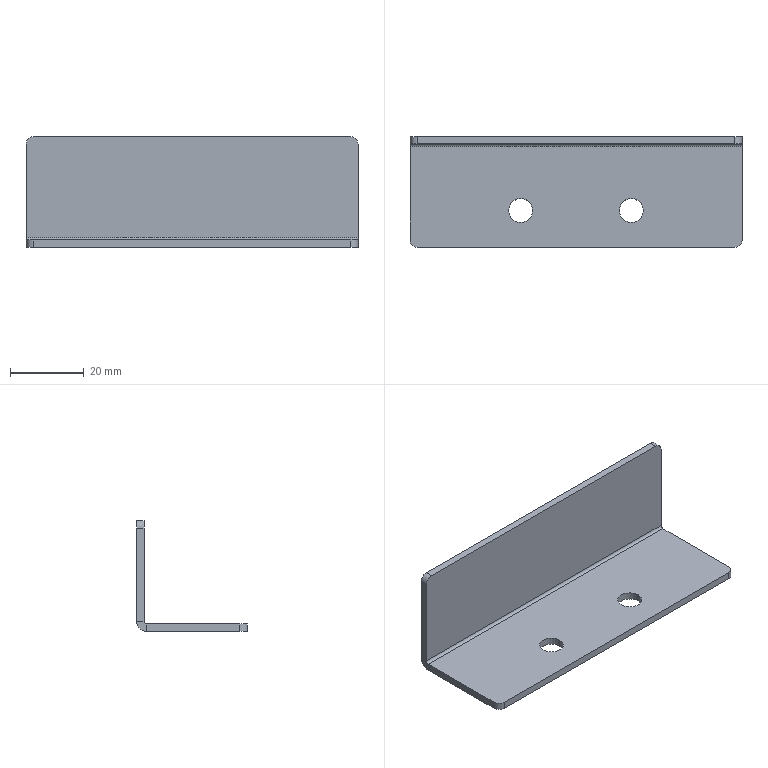Part | STEP file | 02-20 scrap support plate (Default) | 1 solid | 22 faces | box 90 x 30 x 30 mm | volume 10166 mm3 | plane 12 | cylinder 10 | commonest cylinder face diameters 4 x4 6.5 x4 1.473 x1 5.473 x1
STEP:
#1=CARTESIAN_POINT('',(11.75,-4.,-2.));
#2=VERTEX_POINT('',#1);
#3=CARTESIAN_POINT('',(18.25,-4.,-2.));
#4=VERTEX_POINT('',#3);
#5=CARTESIAN_POINT('',(15.,-4.,-2.));
#6=DIRECTION('',(0.,0.,1.));
#7=DIRECTION('',(1.,0.,0.));
#8=AXIS2_PLACEMENT_3D('',#5,#6,#7);
#9=CIRCLE('',#8,3.25);
#10=EDGE_CURVE('',#2,#4,#9,.T.);
#11=ORIENTED_EDGE('',*,*,#10,.F.);
#12=CARTESIAN_POINT('',(11.75,-4.,0.));
#13=VERTEX_POINT('',#12);
#14=CARTESIAN_POINT('',(11.75,-4.,-10.));
#15=DIRECTION('',(0.,0.,1.));
#16=VECTOR('',#15,1000.);
#17=LINE('',#14,#16);
#18=EDGE_CURVE('',#2,#13,#17,.T.);
#19=ORIENTED_EDGE('',*,*,#18,.T.);
#20=CARTESIAN_POINT('',(18.25,-4.,0.));
#21=VERTEX_POINT('',#20);
#22=CARTESIAN_POINT('',(15.,-4.,0.));
#23=DIRECTION('',(0.,0.,1.));
#24=DIRECTION('',(1.,0.,0.));
#25=AXIS2_PLACEMENT_3D('',#22,#23,#24);
#26=CIRCLE('',#25,3.25);
#27=EDGE_CURVE('',#13,#21,#26,.T.);
#28=ORIENTED_EDGE('',*,*,#27,.T.);
#29=CARTESIAN_POINT('',(18.25,-4.,-10.));
#30=DIRECTION('',(0.,0.,1.));
#31=VECTOR('',#30,1000.);
#32=LINE('',#29,#31);
#33=EDGE_CURVE('',#4,#21,#32,.T.);
#34=ORIENTED_EDGE('',*,*,#33,.F.);
#35=EDGE_LOOP('',(#11,#19,#28,#34));
#36=FACE_OUTER_BOUND('',#35,.T.);
#37=CARTESIAN_POINT('',(15.,-4.,-10.));
#38=DIRECTION('',(0.,0.,1.));
#39=DIRECTION('',(1.,0.,0.));
#40=AXIS2_PLACEMENT_3D('',#37,#38,#39);
#41=CYLINDRICAL_SURFACE('',#40,3.25);
#42=ADVANCED_FACE('',(#36),#41,.F.);
#43=CARTESIAN_POINT('',(-18.25,-4.,-2.));
#44=VERTEX_POINT('',#43);
#45=CARTESIAN_POINT('',(-11.75,-4.,-2.));
#46=VERTEX_POINT('',#45);
#47=CARTESIAN_POINT('',(-15.,-4.,-2.));
#48=DIRECTION('',(0.,0.,1.));
#49=DIRECTION('',(1.,0.,0.));
#50=AXIS2_PLACEMENT_3D('',#47,#48,#49);
#51=CIRCLE('',#50,3.25);
#52=EDGE_CURVE('',#44,#46,#51,.T.);
#53=ORIENTED_EDGE('',*,*,#52,.F.);
#54=CARTESIAN_POINT('',(-18.25,-4.,0.));
#55=VERTEX_POINT('',#54);
#56=CARTESIAN_POINT('',(-18.25,-4.,-10.));
#57=DIRECTION('',(0.,0.,1.));
#58=VECTOR('',#57,1000.);
#59=LINE('',#56,#58);
#60=EDGE_CURVE('',#44,#55,#59,.T.);
#61=ORIENTED_EDGE('',*,*,#60,.T.);
#62=CARTESIAN_POINT('',(-11.75,-4.,0.));
#63=VERTEX_POINT('',#62);
#64=CARTESIAN_POINT('',(-15.,-4.,0.));
#65=DIRECTION('',(0.,0.,1.));
#66=DIRECTION('',(1.,0.,0.));
#67=AXIS2_PLACEMENT_3D('',#64,#65,#66);
#68=CIRCLE('',#67,3.25);
#69=EDGE_CURVE('',#55,#63,#68,.T.);
#70=ORIENTED_EDGE('',*,*,#69,.T.);
#71=CARTESIAN_POINT('',(-11.75,-4.,-10.));
#72=DIRECTION('',(0.,0.,1.));
#73=VECTOR('',#72,1000.);
#74=LINE('',#71,#73);
#75=EDGE_CURVE('',#46,#63,#74,.T.);
#76=ORIENTED_EDGE('',*,*,#75,.F.);
#77=EDGE_LOOP('',(#53,#61,#70,#76));
#78=FACE_OUTER_BOUND('',#77,.T.);
#79=CARTESIAN_POINT('',(-15.,-4.,-10.));
#80=DIRECTION('',(0.,0.,1.));
#81=DIRECTION('',(1.,0.,0.));
#82=AXIS2_PLACEMENT_3D('',#79,#80,#81);
#83=CYLINDRICAL_SURFACE('',#82,3.25);
#84=ADVANCED_FACE('',(#78),#83,.F.);
#85=CARTESIAN_POINT('',(-45.,13.263,-2.));
#86=VERTEX_POINT('',#85);
#87=CARTESIAN_POINT('',(-45.,-12.,-2.));
#88=VERTEX_POINT('',#87);
#89=CARTESIAN_POINT('',(-45.,14.,-2.));
#90=DIRECTION('',(0.,-1.,0.));
#91=VECTOR('',#90,1000.);
#92=LINE('',#89,#91);
#93=EDGE_CURVE('',#86,#88,#92,.T.);
#94=ORIENTED_EDGE('',*,*,#93,.T.);
#95=CARTESIAN_POINT('',(-45.,-12.,0.));
#96=VERTEX_POINT('',#95);
#97=CARTESIAN_POINT('',(-45.,-12.,-2.));
#98=DIRECTION('',(0.,0.,1.));
#99=VECTOR('',#98,1000.);
#100=LINE('',#97,#99);
#101=EDGE_CURVE('',#88,#96,#100,.T.);
#102=ORIENTED_EDGE('',*,*,#101,.T.);
#103=CARTESIAN_POINT('',(-45.,13.263,0.));
#104=VERTEX_POINT('',#103);
#105=CARTESIAN_POINT('',(-45.,14.,0.));
#106=DIRECTION('',(0.,-1.,0.));
#107=VECTOR('',#106,1000.);
#108=LINE('',#105,#107);
#109=EDGE_CURVE('',#104,#96,#108,.T.);
#110=ORIENTED_EDGE('',*,*,#109,.F.);
#111=CARTESIAN_POINT('',(-45.,13.263,0.));
#112=DIRECTION('',(0.,0.,-1.));
#113=VECTOR('',#112,1000.);
#114=LINE('',#111,#113);
#115=EDGE_CURVE('',#104,#86,#114,.T.);
#116=ORIENTED_EDGE('',*,*,#115,.T.);
#117=EDGE_LOOP('',(#94,#102,#110,#116));
#118=FACE_OUTER_BOUND('',#117,.T.);
#119=CARTESIAN_POINT('',(-45.,14.,-2.));
#120=DIRECTION('',(-1.,0.,0.));
#121=DIRECTION('',(0.,-1.,0.));
#122=AXIS2_PLACEMENT_3D('',#119,#120,#121);
#123=PLANE('',#122);
#124=ADVANCED_FACE('',(#118),#123,.T.);
#125=CARTESIAN_POINT('',(15.,-4.,-2.));
#126=DIRECTION('',(0.,0.,1.));
#127=DIRECTION('',(1.,0.,0.));
#128=AXIS2_PLACEMENT_3D('',#125,#126,#127);
#129=CIRCLE('',#128,3.25);
#130=EDGE_CURVE('',#4,#2,#129,.T.);
#131=ORIENTED_EDGE('',*,*,#130,.T.);
#132=ORIENTED_EDGE('',*,*,#10,.T.);
#133=EDGE_LOOP('',(#131,#132));
#134=FACE_BOUND('',#133,.T.);
#135=CARTESIAN_POINT('',(-15.,-4.,-2.));
#136=DIRECTION('',(0.,0.,1.));
#137=DIRECTION('',(1.,0.,0.));
#138=AXIS2_PLACEMENT_3D('',#135,#136,#137);
#139=CIRCLE('',#138,3.25);
#140=EDGE_CURVE('',#46,#44,#139,.T.);
#141=ORIENTED_EDGE('',*,*,#140,.T.);
#142=ORIENTED_EDGE('',*,*,#52,.T.);
#143=EDGE_LOOP('',(#141,#142));
#144=FACE_BOUND('',#143,.T.);
#145=CARTESIAN_POINT('',(45.,-12.,-2.));
#146=VERTEX_POINT('',#145);
#147=CARTESIAN_POINT('',(45.,13.263,-2.));
#148=VERTEX_POINT('',#147);
#149=CARTESIAN_POINT('',(45.,14.,-2.));
#150=DIRECTION('',(0.,1.,0.));
#151=VECTOR('',#150,1000.);
#152=LINE('',#149,#151);
#153=EDGE_CURVE('',#146,#148,#152,.T.);
#154=ORIENTED_EDGE('',*,*,#153,.F.);
#155=CARTESIAN_POINT('',(43.,-14.,-2.));
#156=VERTEX_POINT('',#155);
#157=CARTESIAN_POINT('',(43.,-12.,-2.));
#158=DIRECTION('',(0.,0.,-1.));
#159=DIRECTION('',(1.,0.,0.));
#160=AXIS2_PLACEMENT_3D('',#157,#158,#159);
#161=CIRCLE('',#160,2.);
#162=EDGE_CURVE('',#146,#156,#161,.T.);
#163=ORIENTED_EDGE('',*,*,#162,.T.);
#164=CARTESIAN_POINT('',(-43.,-14.,-2.));
#165=VERTEX_POINT('',#164);
#166=CARTESIAN_POINT('',(-45.,-14.,-2.));
#167=DIRECTION('',(1.,0.,0.));
#168=VECTOR('',#167,1000.);
#169=LINE('',#166,#168);
#170=EDGE_CURVE('',#165,#156,#169,.T.);
#171=ORIENTED_EDGE('',*,*,#170,.F.);
#172=CARTESIAN_POINT('',(-43.,-12.,-2.));
#173=DIRECTION('',(0.,0.,-1.));
#174=DIRECTION('',(1.,0.,0.));
#175=AXIS2_PLACEMENT_3D('',#172,#173,#174);
#176=CIRCLE('',#175,2.);
#177=EDGE_CURVE('',#165,#88,#176,.T.);
#178=ORIENTED_EDGE('',*,*,#177,.T.);
#179=ORIENTED_EDGE('',*,*,#93,.F.);
#180=CARTESIAN_POINT('',(-45.,13.263,-2.));
#181=DIRECTION('',(1.,0.,0.));
#182=VECTOR('',#181,1000.);
#183=LINE('',#180,#182);
#184=EDGE_CURVE('',#86,#148,#183,.T.);
#185=ORIENTED_EDGE('',*,*,#184,.T.);
#186=EDGE_LOOP('',(#154,#163,#171,#178,#179,#185));
#187=FACE_OUTER_BOUND('',#186,.T.);
#188=CARTESIAN_POINT('',(45.,-14.,-2.));
#189=DIRECTION('',(0.,0.,1.));
#190=DIRECTION('',(1.,0.,0.));
#191=AXIS2_PLACEMENT_3D('',#188,#189,#190);
#192=PLANE('',#191);
#193=ADVANCED_FACE('',(#134,#144,#187),#192,.F.);
#194=CARTESIAN_POINT('',(15.,-4.,0.));
#195=DIRECTION('',(0.,0.,1.));
#196=DIRECTION('',(1.,0.,0.));
#197=AXIS2_PLACEMENT_3D('',#194,#195,#196);
#198=CIRCLE('',#197,3.25);
#199=EDGE_CURVE('',#21,#13,#198,.T.);
#200=ORIENTED_EDGE('',*,*,#199,.F.);
#201=ORIENTED_EDGE('',*,*,#27,.F.);
#202=EDGE_LOOP('',(#200,#201));
#203=FACE_BOUND('',#202,.T.);
#204=CARTESIAN_POINT('',(-15.,-4.,0.));
#205=DIRECTION('',(0.,0.,1.));
#206=DIRECTION('',(1.,0.,0.));
#207=AXIS2_PLACEMENT_3D('',#204,#205,#206);
#208=CIRCLE('',#207,3.25);
#209=EDGE_CURVE('',#63,#55,#208,.T.);
#210=ORIENTED_EDGE('',*,*,#209,.F.);
#211=ORIENTED_EDGE('',*,*,#69,.F.);
#212=EDGE_LOOP('',(#210,#211));
#213=FACE_BOUND('',#212,.T.);
#214=CARTESIAN_POINT('',(-43.,-14.,0.));
#215=VERTEX_POINT('',#214);
#216=CARTESIAN_POINT('',(43.,-14.,0.));
#217=VERTEX_POINT('',#216);
#218=CARTESIAN_POINT('',(-45.,-14.,0.));
#219=DIRECTION('',(1.,0.,0.));
#220=VECTOR('',#219,1000.);
#221=LINE('',#218,#220);
#222=EDGE_CURVE('',#215,#217,#221,.T.);
#223=ORIENTED_EDGE('',*,*,#222,.T.);
#224=CARTESIAN_POINT('',(45.,-12.,0.));
#225=VERTEX_POINT('',#224);
#226=CARTESIAN_POINT('',(43.,-12.,0.));
#227=DIRECTION('',(0.,0.,1.));
#228=DIRECTION('',(1.,0.,0.));
#229=AXIS2_PLACEMENT_3D('',#226,#227,#228);
#230=CIRCLE('',#229,2.);
#231=EDGE_CURVE('',#217,#225,#230,.T.);
#232=ORIENTED_EDGE('',*,*,#231,.T.);
#233=CARTESIAN_POINT('',(45.,13.263,0.));
#234=VERTEX_POINT('',#233);
#235=CARTESIAN_POINT('',(45.,14.,0.));
#236=DIRECTION('',(0.,1.,0.));
#237=VECTOR('',#236,1000.);
#238=LINE('',#235,#237);
#239=EDGE_CURVE('',#225,#234,#238,.T.);
#240=ORIENTED_EDGE('',*,*,#239,.T.);
#241=CARTESIAN_POINT('',(-45.,13.263,0.));
#242=DIRECTION('',(1.,0.,0.));
#243=VECTOR('',#242,1000.);
#244=LINE('',#241,#243);
#245=EDGE_CURVE('',#104,#234,#244,.T.);
#246=ORIENTED_EDGE('',*,*,#245,.F.);
#247=ORIENTED_EDGE('',*,*,#109,.T.);
#248=CARTESIAN_POINT('',(-43.,-12.,0.));
#249=DIRECTION('',(0.,0.,1.));
#250=DIRECTION('',(1.,0.,0.));
#251=AXIS2_PLACEMENT_3D('',#248,#249,#250);
#252=CIRCLE('',#251,2.);
#253=EDGE_CURVE('',#96,#215,#252,.T.);
#254=ORIENTED_EDGE('',*,*,#253,.T.);
#255=EDGE_LOOP('',(#223,#232,#240,#246,#247,#254));
#256=FACE_OUTER_BOUND('',#255,.T.);
#257=CARTESIAN_POINT('',(45.,-14.,0.));
#258=DIRECTION('',(0.,0.,1.));
#259=DIRECTION('',(1.,0.,0.));
#260=AXIS2_PLACEMENT_3D('',#257,#258,#259);
#261=PLANE('',#260);
#262=ADVANCED_FACE('',(#203,#213,#256),#261,.T.);
#263=ORIENTED_EDGE('',*,*,#239,.F.);
#264=CARTESIAN_POINT('',(45.,-12.,-2.));
#265=DIRECTION('',(0.,0.,-1.));
#266=VECTOR('',#265,1000.);
#267=LINE('',#264,#266);
#268=EDGE_CURVE('',#225,#146,#267,.T.);
#269=ORIENTED_EDGE('',*,*,#268,.T.);
#270=ORIENTED_EDGE('',*,*,#153,.T.);
#271=CARTESIAN_POINT('',(45.,13.263,0.));
#272=DIRECTION('',(0.,0.,-1.));
#273=VECTOR('',#272,1000.);
#274=LINE('',#271,#273);
#275=EDGE_CURVE('',#234,#148,#274,.T.);
#276=ORIENTED_EDGE('',*,*,#275,.F.);
#277=EDGE_LOOP('',(#263,#269,#270,#276));
#278=FACE_OUTER_BOUND('',#277,.T.);
#279=CARTESIAN_POINT('',(45.,14.,-2.));
#280=DIRECTION('',(1.,0.,0.));
#281=DIRECTION('',(0.,0.,-1.));
#282=AXIS2_PLACEMENT_3D('',#279,#280,#281);
#283=PLANE('',#282);
#284=ADVANCED_FACE('',(#278),#283,.T.);
#285=ORIENTED_EDGE('',*,*,#170,.T.);
#286=CARTESIAN_POINT('',(43.,-14.,-2.));
#287=DIRECTION('',(0.,0.,1.));
#288=VECTOR('',#287,1000.);
#289=LINE('',#286,#288);
#290=EDGE_CURVE('',#156,#217,#289,.T.);
#291=ORIENTED_EDGE('',*,*,#290,.T.);
#292=ORIENTED_EDGE('',*,*,#222,.F.);
#293=CARTESIAN_POINT('',(-43.,-14.,-2.));
#294=DIRECTION('',(0.,0.,-1.));
#295=VECTOR('',#294,1000.);
#296=LINE('',#293,#295);
#297=EDGE_CURVE('',#215,#165,#296,.T.);
#298=ORIENTED_EDGE('',*,*,#297,.T.);
#299=EDGE_LOOP('',(#285,#291,#292,#298));
#300=FACE_OUTER_BOUND('',#299,.T.);
#301=CARTESIAN_POINT('',(-45.,-14.,-2.));
#302=DIRECTION('',(0.,-1.,0.));
#303=DIRECTION('',(0.,0.,-1.));
#304=AXIS2_PLACEMENT_3D('',#301,#302,#303);
#305=PLANE('',#304);
#306=ADVANCED_FACE('',(#300),#305,.T.);
#307=CARTESIAN_POINT('',(45.,14.,0.7366));
#308=VERTEX_POINT('',#307);
#309=CARTESIAN_POINT('',(45.,16.,0.7366));
#310=VERTEX_POINT('',#309);
#311=CARTESIAN_POINT('',(45.,14.,0.7366));
#312=DIRECTION('',(0.,1.,0.));
#313=VECTOR('',#312,1000.);
#314=LINE('',#311,#313);
#315=EDGE_CURVE('',#308,#310,#314,.T.);
#316=ORIENTED_EDGE('',*,*,#315,.F.);
#317=CARTESIAN_POINT('',(45.,13.263,0.7366));
#318=DIRECTION('',(1.,0.,0.));
#319=DIRECTION('',(0.,0.,1.));
#320=AXIS2_PLACEMENT_3D('',#317,#318,#319);
#321=CIRCLE('',#320,0.7366);
#322=EDGE_CURVE('',#234,#308,#321,.T.);
#323=ORIENTED_EDGE('',*,*,#322,.F.);
#324=ORIENTED_EDGE('',*,*,#275,.T.);
#325=CARTESIAN_POINT('',(45.,13.263,0.7366));
#326=DIRECTION('',(1.,0.,0.));
#327=DIRECTION('',(0.,0.,1.));
#328=AXIS2_PLACEMENT_3D('',#325,#326,#327);
#329=CIRCLE('',#328,2.737);
#330=EDGE_CURVE('',#148,#310,#329,.T.);
#331=ORIENTED_EDGE('',*,*,#330,.T.);
#332=EDGE_LOOP('',(#316,#323,#324,#331));
#333=FACE_OUTER_BOUND('',#332,.T.);
#334=CARTESIAN_POINT('',(45.,13.263,0.7366));
#335=DIRECTION('',(1.,0.,0.));
#336=DIRECTION('',(0.,0.,-1.));
#337=AXIS2_PLACEMENT_3D('',#334,#335,#336);
#338=PLANE('',#337);
#339=ADVANCED_FACE('',(#333),#338,.T.);
#340=CARTESIAN_POINT('',(-45.,14.,0.7366));
#341=VERTEX_POINT('',#340);
#342=CARTESIAN_POINT('',(-45.,13.263,0.7366));
#343=DIRECTION('',(-1.,0.,0.));
#344=DIRECTION('',(0.,0.,1.));
#345=AXIS2_PLACEMENT_3D('',#342,#343,#344);
#346=CIRCLE('',#345,0.7366);
#347=EDGE_CURVE('',#341,#104,#346,.T.);
#348=ORIENTED_EDGE('',*,*,#347,.F.);
#349=CARTESIAN_POINT('',(-45.,16.,0.7366));
#350=VERTEX_POINT('',#349);
#351=CARTESIAN_POINT('',(-45.,14.,0.7366));
#352=DIRECTION('',(0.,1.,0.));
#353=VECTOR('',#352,1000.);
#354=LINE('',#351,#353);
#355=EDGE_CURVE('',#341,#350,#354,.T.);
#356=ORIENTED_EDGE('',*,*,#355,.T.);
#357=CARTESIAN_POINT('',(-45.,13.263,0.7366));
#358=DIRECTION('',(-1.,0.,0.));
#359=DIRECTION('',(0.,0.,1.));
#360=AXIS2_PLACEMENT_3D('',#357,#358,#359);
#361=CIRCLE('',#360,2.737);
#362=EDGE_CURVE('',#350,#86,#361,.T.);
#363=ORIENTED_EDGE('',*,*,#362,.T.);
#364=ORIENTED_EDGE('',*,*,#115,.F.);
#365=EDGE_LOOP('',(#348,#356,#363,#364));
#366=FACE_OUTER_BOUND('',#365,.T.);
#367=CARTESIAN_POINT('',(-45.,13.263,0.7366));
#368=DIRECTION('',(1.,0.,0.));
#369=DIRECTION('',(0.,0.,-1.));
#370=AXIS2_PLACEMENT_3D('',#367,#368,#369);
#371=PLANE('',#370);
#372=ADVANCED_FACE('',(#366),#371,.F.);
#373=ORIENTED_EDGE('',*,*,#184,.F.);
#374=ORIENTED_EDGE('',*,*,#362,.F.);
#375=CARTESIAN_POINT('',(-45.,16.,0.7366));
#376=DIRECTION('',(-1.,0.,0.));
#377=VECTOR('',#376,1000.);
#378=LINE('',#375,#377);
#379=EDGE_CURVE('',#310,#350,#378,.T.);
#380=ORIENTED_EDGE('',*,*,#379,.F.);
#381=ORIENTED_EDGE('',*,*,#330,.F.);
#382=EDGE_LOOP('',(#373,#374,#380,#381));
#383=FACE_OUTER_BOUND('',#382,.T.);
#384=CARTESIAN_POINT('',(-45.,13.263,0.7366));
#385=DIRECTION('',(-1.,0.,0.));
#386=DIRECTION('',(0.,1.,0.));
#387=AXIS2_PLACEMENT_3D('',#384,#385,#386);
#388=CYLINDRICAL_SURFACE('',#387,2.737);
#389=ADVANCED_FACE('',(#383),#388,.T.);
#390=ORIENTED_EDGE('',*,*,#245,.T.);
#391=ORIENTED_EDGE('',*,*,#322,.T.);
#392=CARTESIAN_POINT('',(45.,14.,0.7366));
#393=DIRECTION('',(-1.,0.,0.));
#394=VECTOR('',#393,1000.);
#395=LINE('',#392,#394);
#396=EDGE_CURVE('',#308,#341,#395,.T.);
#397=ORIENTED_EDGE('',*,*,#396,.T.);
#398=ORIENTED_EDGE('',*,*,#347,.T.);
#399=EDGE_LOOP('',(#390,#391,#397,#398));
#400=FACE_OUTER_BOUND('',#399,.T.);
#401=CARTESIAN_POINT('',(-45.,13.263,0.7366));
#402=DIRECTION('',(-1.,0.,0.));
#403=DIRECTION('',(0.,1.,0.));
#404=AXIS2_PLACEMENT_3D('',#401,#402,#403);
#405=CYLINDRICAL_SURFACE('',#404,0.7366);
#406=ADVANCED_FACE('',(#400),#405,.F.);
#407=CARTESIAN_POINT('',(-45.,14.,26.));
#408=VERTEX_POINT('',#407);
#409=CARTESIAN_POINT('',(-45.,14.,0.));
#410=DIRECTION('',(0.,0.,-1.));
#411=VECTOR('',#410,1000.);
#412=LINE('',#409,#411);
#413=EDGE_CURVE('',#408,#341,#412,.T.);
#414=ORIENTED_EDGE('',*,*,#413,.F.);
#415=CARTESIAN_POINT('',(-45.,16.,26.));
#416=VERTEX_POINT('',#415);
#417=CARTESIAN_POINT('',(-45.,16.,26.));
#418=DIRECTION('',(0.,1.,0.));
#419=VECTOR('',#418,1000.);
#420=LINE('',#417,#419);
#421=EDGE_CURVE('',#408,#416,#420,.T.);
#422=ORIENTED_EDGE('',*,*,#421,.T.);
#423=CARTESIAN_POINT('',(-45.,16.,0.));
#424=DIRECTION('',(0.,0.,-1.));
#425=VECTOR('',#424,1000.);
#426=LINE('',#423,#425);
#427=EDGE_CURVE('',#416,#350,#426,.T.);
#428=ORIENTED_EDGE('',*,*,#427,.T.);
#429=ORIENTED_EDGE('',*,*,#355,.F.);
#430=EDGE_LOOP('',(#414,#422,#428,#429));
#431=FACE_OUTER_BOUND('',#430,.T.);
#432=CARTESIAN_POINT('',(-45.,16.,0.));
#433=DIRECTION('',(-1.,0.,0.));
#434=DIRECTION('',(0.,0.,1.));
#435=AXIS2_PLACEMENT_3D('',#432,#433,#434);
#436=PLANE('',#435);
#437=ADVANCED_FACE('',(#431),#436,.T.);
#438=CARTESIAN_POINT('',(45.,16.,26.));
#439=VERTEX_POINT('',#438);
#440=CARTESIAN_POINT('',(45.,16.,28.));
#441=DIRECTION('',(0.,0.,1.));
#442=VECTOR('',#441,1000.);
#443=LINE('',#440,#442);
#444=EDGE_CURVE('',#310,#439,#443,.T.);
#445=ORIENTED_EDGE('',*,*,#444,.T.);
#446=CARTESIAN_POINT('',(45.,14.,26.));
#447=VERTEX_POINT('',#446);
#448=CARTESIAN_POINT('',(45.,16.,26.));
#449=DIRECTION('',(0.,-1.,0.));
#450=VECTOR('',#449,1000.);
#451=LINE('',#448,#450);
#452=EDGE_CURVE('',#439,#447,#451,.T.);
#453=ORIENTED_EDGE('',*,*,#452,.T.);
#454=CARTESIAN_POINT('',(45.,14.,28.));
#455=DIRECTION('',(0.,0.,1.));
#456=VECTOR('',#455,1000.);
#457=LINE('',#454,#456);
#458=EDGE_CURVE('',#308,#447,#457,.T.);
#459=ORIENTED_EDGE('',*,*,#458,.F.);
#460=ORIENTED_EDGE('',*,*,#315,.T.);
#461=EDGE_LOOP('',(#445,#453,#459,#460));
#462=FACE_OUTER_BOUND('',#461,.T.);
#463=CARTESIAN_POINT('',(45.,16.,28.));
#464=DIRECTION('',(1.,0.,0.));
#465=DIRECTION('',(0.,0.,-1.));
#466=AXIS2_PLACEMENT_3D('',#463,#464,#465);
#467=PLANE('',#466);
#468=ADVANCED_FACE('',(#462),#467,.T.);
#469=CARTESIAN_POINT('',(43.,16.,28.));
#470=VERTEX_POINT('',#469);
#471=CARTESIAN_POINT('',(-43.,16.,28.));
#472=VERTEX_POINT('',#471);
#473=CARTESIAN_POINT('',(-45.,16.,28.));
#474=DIRECTION('',(-1.,0.,0.));
#475=VECTOR('',#474,1000.);
#476=LINE('',#473,#475);
#477=EDGE_CURVE('',#470,#472,#476,.T.);
#478=ORIENTED_EDGE('',*,*,#477,.F.);
#479=CARTESIAN_POINT('',(43.,16.,26.));
#480=DIRECTION('',(0.,1.,0.));
#481=DIRECTION('',(0.,0.,1.));
#482=AXIS2_PLACEMENT_3D('',#479,#480,#481);
#483=CIRCLE('',#482,2.);
#484=EDGE_CURVE('',#470,#439,#483,.T.);
#485=ORIENTED_EDGE('',*,*,#484,.T.);
#486=ORIENTED_EDGE('',*,*,#444,.F.);
#487=ORIENTED_EDGE('',*,*,#379,.T.);
#488=ORIENTED_EDGE('',*,*,#427,.F.);
#489=CARTESIAN_POINT('',(-43.,16.,26.));
#490=DIRECTION('',(0.,1.,0.));
#491=DIRECTION('',(0.,0.,1.));
#492=AXIS2_PLACEMENT_3D('',#489,#490,#491);
#493=CIRCLE('',#492,2.);
#494=EDGE_CURVE('',#416,#472,#493,.T.);
#495=ORIENTED_EDGE('',*,*,#494,.T.);
#496=EDGE_LOOP('',(#478,#485,#486,#487,#488,#495));
#497=FACE_OUTER_BOUND('',#496,.T.);
#498=CARTESIAN_POINT('',(-45.,16.,0.));
#499=DIRECTION('',(0.,1.,0.));
#500=DIRECTION('',(0.,0.,1.));
#501=AXIS2_PLACEMENT_3D('',#498,#499,#500);
#502=PLANE('',#501);
#503=ADVANCED_FACE('',(#497),#502,.T.);
#504=ORIENTED_EDGE('',*,*,#458,.T.);
#505=CARTESIAN_POINT('',(43.,14.,28.));
#506=VERTEX_POINT('',#505);
#507=CARTESIAN_POINT('',(43.,14.,26.));
#508=DIRECTION('',(0.,-1.,0.));
#509=DIRECTION('',(0.,0.,1.));
#510=AXIS2_PLACEMENT_3D('',#507,#508,#509);
#511=CIRCLE('',#510,2.);
#512=EDGE_CURVE('',#447,#506,#511,.T.);
#513=ORIENTED_EDGE('',*,*,#512,.T.);
#514=CARTESIAN_POINT('',(-43.,14.,28.));
#515=VERTEX_POINT('',#514);
#516=CARTESIAN_POINT('',(-45.,14.,28.));
#517=DIRECTION('',(-1.,0.,0.));
#518=VECTOR('',#517,1000.);
#519=LINE('',#516,#518);
#520=EDGE_CURVE('',#506,#515,#519,.T.);
#521=ORIENTED_EDGE('',*,*,#520,.T.);
#522=CARTESIAN_POINT('',(-43.,14.,26.));
#523=DIRECTION('',(0.,-1.,0.));
#524=DIRECTION('',(0.,0.,1.));
#525=AXIS2_PLACEMENT_3D('',#522,#523,#524);
#526=CIRCLE('',#525,2.);
#527=EDGE_CURVE('',#515,#408,#526,.T.);
#528=ORIENTED_EDGE('',*,*,#527,.T.);
#529=ORIENTED_EDGE('',*,*,#413,.T.);
#530=ORIENTED_EDGE('',*,*,#396,.F.);
#531=EDGE_LOOP('',(#504,#513,#521,#528,#529,#530));
#532=FACE_OUTER_BOUND('',#531,.T.);
#533=CARTESIAN_POINT('',(-45.,14.,0.));
#534=DIRECTION('',(0.,1.,0.));
#535=DIRECTION('',(0.,0.,1.));
#536=AXIS2_PLACEMENT_3D('',#533,#534,#535);
#537=PLANE('',#536);
#538=ADVANCED_FACE('',(#532),#537,.F.);
#539=ORIENTED_EDGE('',*,*,#520,.F.);
#540=CARTESIAN_POINT('',(43.,16.,28.));
#541=DIRECTION('',(0.,1.,0.));
#542=VECTOR('',#541,1000.);
#543=LINE('',#540,#542);
#544=EDGE_CURVE('',#506,#470,#543,.T.);
#545=ORIENTED_EDGE('',*,*,#544,.T.);
#546=ORIENTED_EDGE('',*,*,#477,.T.);
#547=CARTESIAN_POINT('',(-43.,16.,28.));
#548=DIRECTION('',(0.,-1.,0.));
#549=VECTOR('',#548,1000.);
#550=LINE('',#547,#549);
#551=EDGE_CURVE('',#472,#515,#550,.T.);
#552=ORIENTED_EDGE('',*,*,#551,.T.);
#553=EDGE_LOOP('',(#539,#545,#546,#552));
#554=FACE_OUTER_BOUND('',#553,.T.);
#555=CARTESIAN_POINT('',(-45.,16.,28.));
#556=DIRECTION('',(0.,0.,1.));
#557=DIRECTION('',(0.,-1.,0.));
#558=AXIS2_PLACEMENT_3D('',#555,#556,#557);
#559=PLANE('',#558);
#560=ADVANCED_FACE('',(#554),#559,.T.);
#561=ORIENTED_EDGE('',*,*,#162,.F.);
#562=ORIENTED_EDGE('',*,*,#268,.F.);
#563=ORIENTED_EDGE('',*,*,#231,.F.);
#564=ORIENTED_EDGE('',*,*,#290,.F.);
#565=EDGE_LOOP('',(#561,#562,#563,#564));
#566=FACE_OUTER_BOUND('',#565,.T.);
#567=CARTESIAN_POINT('',(43.,-12.,-2.));
#568=DIRECTION('',(0.,0.,1.));
#569=DIRECTION('',(1.,0.,0.));
#570=AXIS2_PLACEMENT_3D('',#567,#568,#569);
#571=CYLINDRICAL_SURFACE('',#570,2.);
#572=ADVANCED_FACE('',(#566),#571,.T.);
#573=ORIENTED_EDGE('',*,*,#484,.F.);
#574=ORIENTED_EDGE('',*,*,#544,.F.);
#575=ORIENTED_EDGE('',*,*,#512,.F.);
#576=ORIENTED_EDGE('',*,*,#452,.F.);
#577=EDGE_LOOP('',(#573,#574,#575,#576));
#578=FACE_OUTER_BOUND('',#577,.T.);
#579=CARTESIAN_POINT('',(43.,16.,26.));
#580=DIRECTION('',(0.,-1.,0.));
#581=DIRECTION('',(0.,0.,-1.));
#582=AXIS2_PLACEMENT_3D('',#579,#580,#581);
#583=CYLINDRICAL_SURFACE('',#582,2.);
#584=ADVANCED_FACE('',(#578),#583,.T.);
#585=ORIENTED_EDGE('',*,*,#494,.F.);
#586=ORIENTED_EDGE('',*,*,#421,.F.);
#587=ORIENTED_EDGE('',*,*,#527,.F.);
#588=ORIENTED_EDGE('',*,*,#551,.F.);
#589=EDGE_LOOP('',(#585,#586,#587,#588));
#590=FACE_OUTER_BOUND('',#589,.T.);
#591=CARTESIAN_POINT('',(-43.,16.,26.));
#592=DIRECTION('',(0.,-1.,0.));
#593=DIRECTION('',(0.,0.,-1.));
#594=AXIS2_PLACEMENT_3D('',#591,#592,#593);
#595=CYLINDRICAL_SURFACE('',#594,2.);
#596=ADVANCED_FACE('',(#590),#595,.T.);
#597=ORIENTED_EDGE('',*,*,#177,.F.);
#598=ORIENTED_EDGE('',*,*,#297,.F.);
#599=ORIENTED_EDGE('',*,*,#253,.F.);
#600=ORIENTED_EDGE('',*,*,#101,.F.);
#601=EDGE_LOOP('',(#597,#598,#599,#600));
#602=FACE_OUTER_BOUND('',#601,.T.);
#603=CARTESIAN_POINT('',(-43.,-12.,-2.));
#604=DIRECTION('',(0.,0.,1.));
#605=DIRECTION('',(1.,0.,0.));
#606=AXIS2_PLACEMENT_3D('',#603,#604,#605);
#607=CYLINDRICAL_SURFACE('',#606,2.);
#608=ADVANCED_FACE('',(#602),#607,.T.);
#609=ORIENTED_EDGE('',*,*,#60,.F.);
#610=ORIENTED_EDGE('',*,*,#140,.F.);
#611=ORIENTED_EDGE('',*,*,#75,.T.);
#612=ORIENTED_EDGE('',*,*,#209,.T.);
#613=EDGE_LOOP('',(#609,#610,#611,#612));
#614=FACE_OUTER_BOUND('',#613,.T.);
#615=CARTESIAN_POINT('',(-15.,-4.,-10.));
#616=DIRECTION('',(0.,0.,1.));
#617=DIRECTION('',(1.,0.,0.));
#618=AXIS2_PLACEMENT_3D('',#615,#616,#617);
#619=CYLINDRICAL_SURFACE('',#618,3.25);
#620=ADVANCED_FACE('',(#614),#619,.F.);
#621=ORIENTED_EDGE('',*,*,#18,.F.);
#622=ORIENTED_EDGE('',*,*,#130,.F.);
#623=ORIENTED_EDGE('',*,*,#33,.T.);
#624=ORIENTED_EDGE('',*,*,#199,.T.);
#625=EDGE_LOOP('',(#621,#622,#623,#624));
#626=FACE_OUTER_BOUND('',#625,.T.);
#627=CARTESIAN_POINT('',(15.,-4.,-10.));
#628=DIRECTION('',(0.,0.,1.));
#629=DIRECTION('',(1.,0.,0.));
#630=AXIS2_PLACEMENT_3D('',#627,#628,#629);
#631=CYLINDRICAL_SURFACE('',#630,3.25);
#632=ADVANCED_FACE('',(#626),#631,.F.);
#633=CLOSED_SHELL('',(#42,#84,#124,#193,#262,#284,#306,#339,#372,#389,#406,#437,#468,#503,#538,#560,#572,#584,#596,#608,#620,#632));
#634=MANIFOLD_SOLID_BREP('',#633);
#635=CARTESIAN_POINT('',(0.,0.,0.));
#636=DIRECTION('',(0.,0.,1.));
#637=DIRECTION('',(1.,0.,0.));
#638=AXIS2_PLACEMENT_3D('',#635,#636,#637);
#639=(LENGTH_UNIT()NAMED_UNIT(*)SI_UNIT(.MILLI.,.METRE.));
#640=UNCERTAINTY_MEASURE_WITH_UNIT(LENGTH_MEASURE(0.00001),#639,'','');
#641=(NAMED_UNIT(*)PLANE_ANGLE_UNIT()SI_UNIT($,.RADIAN.));
#642=(NAMED_UNIT(*)SI_UNIT($,.STERADIAN.)SOLID_ANGLE_UNIT());
#643=(GEOMETRIC_REPRESENTATION_CONTEXT(3)GLOBAL_UNCERTAINTY_ASSIGNED_CONTEXT((#640))GLOBAL_UNIT_ASSIGNED_CONTEXT((#639,#641,#642))REPRESENTATION_CONTEXT('',''));
#644=ADVANCED_BREP_SHAPE_REPRESENTATION('',(#634,#638),#643);